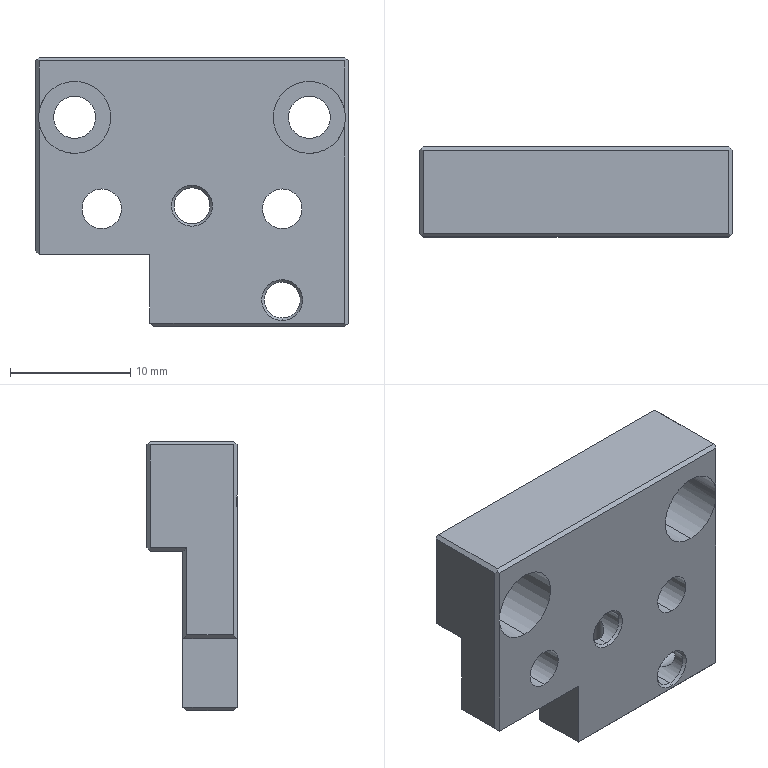Part | NX | 1 solid | 58 faces | box 26 x 7.5 x 22.4 mm | volume 2551 mm3 | plane 30 | cylinder 20 | cone 8 | commonest cylinder face diameters 2.5 x4 3 x4 3.3 x4 3.5 x4 6 x4